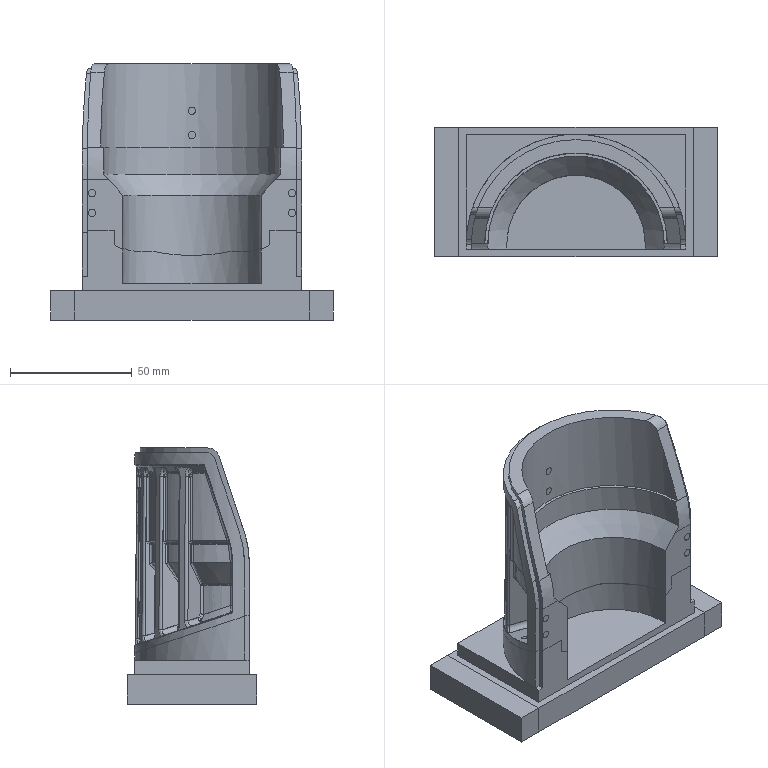NC program | NX | posted by the shop | part box 116 x 53 x 105 mm
Lines 1 to 928 of 572762:
CYCLE800
TRAFOOF
TRANS
ROT
G40 G17 G710 G94 G90 G60 G601 FNORM
TRAFOOF
SUPA G0 Z-1. D0
SUPA G0 X-1.0 Y-1.0
T18 M6
;(T18:C-D10  D=10. R=0.)
;(XY=0.mm Z=0.1mm)
G54 G90 D1
G0 A0.0 C=DC(0.0)
CYCLE832(0.12,_TOP_SURFACE_SMOOTH_ON+_ORI_SEMIFIN,1.)
G0 X54.1 Y-23.625 S7000 M3 M8
Z43.
Z3.1
G94 G1 Z.1 F1500.
X53.
X-53.
Y-15.75
X53.
Y-7.875
X-53.
Y0.0
X53.
Y7.875
X-53.
Y15.75
X53.
Y23.625
X-53.
X-54.1
Z3.1
G0 Z43.
CYCLE832()
;(T18:C-D10  D=10. R=0.)
;(XY=0.3mm Z=0.3mm)
SUPA G0 Z-1. D0
SUPA G0 X-1.0 Y-1.0
G54 G90 D1
CYCLE832(0.32,_ROUGH,1.)
TRAFOOF
CYCLE800(0,"AFMING",100000,57,0.,0.,0.,-90.,0.,-0.,0.,0.,0.,-1,100.,1)
G0 X55.844 Y85.217 S7000 M3
Z67.41
X55.844 Y85.217 Z67.41
Z3.8
G1 Z.8 F3500.
G3 X55.651 Y86.799 I-.713 J.7156
G1 X54.93 Y87.243
X54.186 Y87.648
G3 X52.997 Y87.1846 I-.31 J-.963
X52.447 Y81.73 I20.436 J-4.814
G1 X52.397 Y72.375
X52.369 Y1.951
G2 X48.396 Y-3.028 I-6.274 J.932
X41.431 Y-4.3 I-6.806 J17.567
G3 X39.312 Y-4.464 I-.547 J-6.7
G1 X38.261 Y-4.967
G3 X37.691 Y-6.068 I.414 J-.913
X38.403 Y-6.8609 Z1.081 I1.068 J.243 TURN=0
G1 X39.178 Y-7.242 Z1.3
X40.9306 Y-8.09 F15000.
X41.169 Y-8.126
X41.409 Y-8.116
X43.432 Y-7.734
X45.441 Y-7.287
G3 X48.546 Y-6.223 I-6.272 J23.35
G1 X51.559 Y-4.93
G3 X55.195 Y.607 I-3.082 J5.986
G1 X55.354 Y3.693
X55.433 Y6.781
X56.109 Y84.343
X55.986 Y84.715
X55.727 Y85.171
X54.75 Y86.892 Z.8 F3500.
G3 X54.225 Y87.552 I-1.461 J-.623
X52.968 Y87.361 I-.512 J-.861
X52.003 Y82.98 I9.95 J-4.489
X51.7982 Y72.298 I208.361 J-9.332
G1 X51.776 Y4.15
G2 X46.875 Y-2.259 I-7.688 J.8
X40.862 Y-3.6267 I-7.74 J20.124
G3 X39.209 Y-4.523 I.69 J-3.245
X38.928 Y-5.8101 I.597 J-.805
X39.845 Y-6.345 Z1.08 I.942 J.562 TURN=0
G1 X40.704 Y-6.475 Z1.3
X42.797 Y-6.781 F15000.
X43.0644 Y-6.749
X48.069 Y-5.4272
G3 X51.335 Y-3.4251 I-2.55 J7.826
G1 X52.151 Y-2.616
X52.926 Y-1.767
G3 X54.4545 Y1.9676 I-5.961 J4.62
X54.917 Y8.1208 I-45.709 J6.5262
G1 X55.097 Y83.6231
X54.875 Y85.1759
X54.6051 Y86.983 Z.838 F3500.
X54.55 Y87.124 Z.8
G3 X52.881 Y87.335 I-.903 J-.431
X51.5659 Y83.141 I7.417 J-4.629
X51.199 Y70.723 I125.865 J-9.938
G1 X51.161 Y5.775
G2 X45.553 Y-1.5865 I-8.669 J.787
X41.04 Y-3.01 I-24.116 J68.574
G3 X40.107 Y-3.859 I1.703 J-2.811
X39.802 Y-5.101 I.597 J-.805
X40.692 Y-5.6815 Z1.08 I.969 J.514 TURN=0
G1 X41.543 Y-5.854 Z1.3
X43.403 Y-6.221 F15000.
X43.692 Y-6.191
X43.963 Y-6.085
X49.2849 Y-2.953
G3 X52.679 Y.725 I-6.142 J9.073
X53.789 Y3.142 I-9.965 J6.04
G1 X53.966 Y3.937
X54.05 Y4.748
X54.156 Y7.837
X54.2243 Y10.926
X55.047 Y83.497
X54.802 Y85.18
X54.514 Y86.981 Z.839 F3500.
X54.456 Y87.124 Z.8
G3 X52.821 Y87.353 I-.896 J-.445
X51.177 Y83.411 I5.612 J-4.654
X50.615 Y73.095 I70.0607 J-8.9932
G1 X50.569 Y7.525
G2 X44.815 Y-.77 I-9.467 J.424
G1 X42.844 Y-1.662
G2 X40.805 Y-3.102 I-10.229 J12.317
G1 X40.655 Y-3.27
G3 X40.884 Y-4.794 I.746 J-.667
X41.802 Y-4.895 Z1.039 I.592 J1.162 TURN=0
G1 X42.826 Y-4.768 Z1.3
X44.706 Y-4.526 F15000.
X44.955 Y-4.422
G3 X48.058 Y-2.402 I-11.603 J21.212
G1 X50.369 Y-.546
G3 X52.6816 Y3.133 I-4.852 J5.616
X53.56 Y7.794 I-25.859 J7.289
G1 X53.633 Y9.199
X55.086 Y83.83
X54.7686 Y85.177
X54.288 Y87.0955 Z.8 F3500.
G3 X52.866 Y87.557 I-.917 J-.402
X50.885 Y83.959 I4.201 J-4.656
X50.0605 Y74.984 I42.887 J-8.467
G1 X49.998 Y66.826
X49.9665 Y8.951
G2 X44.667 Y.237 I-10.345 J.323
G3 X43.144 Y-1.352 I1.364 J-2.832
G1 X42.844 Y-1.662
G3 X43.3856 Y-3.342 I.719 J-.695
X44.258 Y-3.132 Z1.031 I.14 J1.335 TURN=0
G1 X45.214 Y-2.669 Z1.3
X46.966 Y-1.821 F15000.
X48.703 Y-.943
G3 X50.137 Y.509 I-2.2007 J3.607
G1 X51.6321 Y3.07
G3 X52.737 Y6.707 I-10.456 J5.162
G1 X52.898 Y8.242
X52.968 Y9.784
X53.953 Y83.3736
X54.083 Y85.165
X54.187 Y86.795 Z.887 F3500.
X54.095 Y87.125 Z.8
G3 X52.798 Y87.615 I-.904 J-.431
X50.563 Y84.212 I3.395 J-4.667
X49.516 Y75.745 I33.271 J-8.412
X49.398 Y63.5248 I611.077 J-11.991
G1 X49.367 Y10.35
G2 X45.447 Y1.972 I-11.0628 J.0696
G3 X44.13 Y.553 I2.872 J-3.987
G2 X43.6261 Y-.568 I-4.072 J1.158
G3 X43.988 Y-1.963 I.853 J-.524
X45.011 Y-1.957 Z1.069 I.506 J.97 TURN=0
G1 X45.8612 Y-1.625 Z1.3
X47.748 Y-.877 F15000.
X47.926 Y-.736
X48.078 Y-.568
X50.408 Y2.93
G3 X52.304 Y9.496 I-12.158 J7.068
G1 X53.771 Y83.349
X53.9585 Y85.177
X54.051 Y85.988 Z1.093 F3500.
X54.101 Y86.803 Z.887
X54.01 Y87.1328 Z.8
G3 X52.614 Y87.567 I-.901 J-.435
X50.225 Y84.351 I2.982 J-4.709
X48.98 Y76.204 I27.997 J-8.45
X48.798 Y62.1 I403.271 J-12.238
G1 X48.767 Y11.65
G2 X45.1621 Y2.856 I-13.09 J.231
G3 X44.293 Y1.462 I2.508 J-2.531
G1 X44.124 Y.529
G3 X44.849 Y-.686 I.971 J-.245
X45.862 Y-.385 Z1.079 I.232 J1.0738 TURN=0
G1 X46.551 Y.153 Z1.3
X48.326 Y1.556 F15000.
G3 X50.309 Y4.865 I-15.901 J11.776
X51.075 Y7.201 I-10.588 J4.766
X51.877 Y13.303 I-28.779 J6.887
G1 X53.01 Y83.391
X53.564 Y85.175
X53.988 Y86.567 Z.932 F3500.
X53.982 Y86.8268 Z.866
X53.922 Y87.08 Z.8
G3 X52.997 Y87.699 I-.927 J-.385
X50.979 Y86.405 I.371 J-2.8
X48.891 Y80.7036 I10.399 J-7.0413
X48.218 Y68.369 I88.071 J-10.989
G1 X48.169 Y12.9258
G2 X45.388 Y4.437 I-14.695 J.114
G3 X44.347 Y2.488 I4.572 J-3.693
G1 X44.292 Y1.444
G3 X44.953 Y.441 I1.001 J-.06
X45.992 Y.644 Z1.079 I.334 J1.046 TURN=0
G1 X46.727 Y1.114 Z1.3
X47.72 Y1.763 F15000.
G3 X48.055 Y2.452 I-.688 J.76
G1 X52.847 Y83.803
X52.913 Y84.106
X53.326 Y85.169
X53.6 Y85.851 Z1.114 F3500.
X53.833 Y86.547 Z.928
X53.837 Y86.8 Z.864
X53.784 Y87.047 Z.8
G3 X52.847 Y87.699 I-.94 J-.352
X50.747 Y86.506 I.228 J-2.847
X49.838 Y84.837 I2.45 J-2.416
X48.1816 Y79.188 I12.972 J-6.872
X47.605 Y65.162 I120.7863 J-11.987
G1 X47.567 Y14.0503
G2 X44.995 Y5.187 I-17.807 J.363
G3 X44.347 Y2.464 I3.144 J-2.187
X45.455 Y1.47 I1.001 J.001
X46.277 Y2.053 Z1.064 I-.158 J1.094 TURN=0
G1 X46.803 Y2.821 Z1.3
X47.6162 Y4.025 F15000.
X47.721 Y4.412
X52.643 Y83.955
X53.102 Y85.17
X53.376 Y85.852 Z1.114 F3500.
X53.608 Y86.548 Z.928
X53.612 Y86.801 Z.864
X53.5589 Y87.049 Z.8
G3 X52.622 Y87.699 I-.939 J-.353
X50.041 Y85.495 I.09 J-2.719
X50.88 Y84.092 I1.052 J-.324
X52.032 Y84.568 Z1.132 I.196 J1.1581 TURN=0
G1 X52.479 Y85.0572 Z1.3
X52.5854 Y85.174 F15000.
X52.991 Y85.607 Z1.15 F3500.
X53.359 Y86.072 Z.999
G3 X53.471 Y86.836 Z.8 I-.986 J.535 TURN=0
X52.397 Y87.699 I-1.076 J-.24
X50.259 Y86.411 I-.086 J-2.276
G1 X50.219 Y86.077
G3 X51.945 Y85.099 I1.0976 J-.075
G1 X52.936 Y85.807
G3 X52.172 Y87.698 I-.764 J.792
X50.25 Y86.536 I-.249 J-1.757
G1 X50.2298 Y86.236
G3 X52.015 Y85.3033 I1.098 J-.0746
G1 X52.691 Y85.864
G3 X51.872 Y87.698 I-.819 J.734
X50.248 Y86.5 I-.27 J-1.333
X52.139 Y87.568 I1.3048 J-.102
X50.313 Y86.986 I-.64 J-1.1444
G2 X48.967 Y83.429 I-6.462 J.4142
G3 X47.484 Y77.555 I14.984 J-6.905
X47.0012 Y62.695 I154.428 J-12.4597
G1 X46.965 Y15.1
G2 X44.635 Y5.965 I-21.638 J.653
G1 X44.347 Y5.098
Y3.598
G3 X46.545 Y3.536 I1.1 J0.
G1 X46.658 Y5.541
X46.769 Y7.517 Z1.3
X50.957 Y81.972 F15000.
X50.9927 Y82.52 Z1.161 F3500.
X50.99 Y83.068 Z1.022
G3 X50.536 Y83.794 Z.8 I-1.098 J-.182 TURN=0
X49.071 Y83.606 I-.628 J-.905
X47.379 Y79.8146 I5.919 J-4.916
X46.475 Y69.356 I56.897 J-10.182
G1 X46.399 Y58.275
X46.359 Y16.0001
G2 X44.364 Y6.962 I-26.36 J1.079
G1 X44.347 Y5.061
G3 X46.545 Y5.001 I1.1 J0.
G1 X46.5974 Y5.961
X46.705 Y7.937 Z1.3
X50.705 Y81.7157 F15000.
X50.739 Y82.264 Z1.161 F3500.
X50.736 Y82.813 Z1.022
G3 X50.282 Y83.537 Z.8 I-1.0978 J-.184 TURN=0
X48.943 Y83.474 I-.628 J-.9055
X47.063 Y80.18 I4.108 J-4.527
X45.938 Y70.643 I40.914 J-9.662
X45.799 Y56.325 I637.665 J-13.3519
G1 X45.758 Y16.975
G2 X44.184 Y8.359 I-31.504 J1.3038
G3 X44.3262 Y7.267 I5.283 J.134
G1 X44.335 Y6.742
G3 X46.472 Y6.393 I1.1 J.019
G1 X46.549 Y6.887 Z.927
X46.568 Y7.387 Z1.053
X46.618 Y8.362 Z1.3
X50.364 Y81.419 F15000.
X50.3966 Y81.971 Z1.16 F3500.
X50.392 Y82.524 Z1.02
G3 X49.943 Y83.243 Z.8 I-1.098 J-.186 TURN=0
X48.5993 Y83.184 I-.634 J-.902
X46.524 Y79.7 I4.14 J-4.826
X45.35 Y70.108 I40.181 J-9.7839
X45.199 Y56.25 I626.297 J-13.752
G1 X45.156 Y17.875
G2 X43.916 Y9.6902 I-38.899 J1.705
G3 X44.075 Y8.504 I1.546 J-.397
G1 X44.18 Y7.989
G3 X45.979 Y7.378 I1.078 J.219
X46.3695 Y8.4274 Z1.092 I-.918 J.939 TURN=0
G1 X46.409 Y9.245 Z1.3
X49.908 Y81.031 F15000.
X49.939 Y81.584 Z1.16 F3500.
X49.934 Y82.138 Z1.0191
G3 X49.486 Y82.855 Z.8 I-1.098 J-.188 TURN=0
X48.141 Y82.796 I-.634 J-.902
X45.9618 Y79.17 I4.266 J-5.032
X44.785 Y69.9959 I39.41 J-9.717
X44.6 Y54.975 I457.94 J-13.17
G1 X44.555 Y18.775
G2 X43.537 Y10.733 I-51.515 J2.439
G3 X43.942 Y8.81 I2.766 J-.422
X45.467 Y8.278 I1.009 J.44
X46.058 Y9.384 Z1.134 I-.578 J1.0195 TURN=0
G1 X46.088 Y10.037 Z1.3
X49.383 Y80.573 F15000.
X49.418 Y81.159 Z1.151 F3500.
X49.402 Y81.7468 Z1.002
G3 X48.988 Y82.412 Z.8 I-1.098 J-.222 TURN=0
X47.769 Y82.481 I-.662 J-.883
X45.723 Y79.622 I2.988 J-4.301
X44.315 Y71.537 I27.9197 J-9.026
X43.999 Y55.351 I273.069 J-13.4202
G1 X43.965 Y19.9759
G2 X43.098 Y11.541 I-74.422 J3.384
G3 X43.5717 Y9.661 I2.158 J-.456
X45.051 Y9.106 I1.009 J.44
X45.689 Y10.244 Z1.15 I-.533 J1.046 TURN=0
G1 X45.7172 Y10.8365 Z1.3
X49.071 Y80.3461 F15000.
X49.107 Y80.953 Z1.146 F3500.
X49.097 Y81.561 Z.992
G3 X48.725 Y82.206 Z.8 I-1.1066 J-.21 TURN=0
X47.588 Y82.375 I-.707 J-.849
X45.462 Y79.892 I2.144 J-3.987
X44.375 Y76.218 I16.1043 J-6.762
G2 X44.302 Y72.5245 I-59.855 J-.66
G3 X43.51 Y65.556 I27.897 J-6.698
G1 X43.429 Y55.97
X43.39 Y22.102
G2 X42.645 Y12.462 I-91.099 J2.188
G3 X42.8445 Y10.67 I3.454 J-.523
G1 X43.291 Y10.067
G3 X44.644 Y9.728 I.884 J.658
X45.2824 Y10.842 Z1.144 I-.52 J1.038 TURN=0
G1 X45.314 Y11.457 Z1.3
X48.86 Y80.24 F15000.
X48.898 Y80.853 Z1.145 F3500.
X48.892 Y81.466 Z.989
G3 X48.531 Y82.106 Z.8 I-1.11 J-.203 TURN=0
X47.3809 Y82.287 I-.721 J-.837
X45.042 Y79.776 I1.919 J-4.134
X44.346 Y77.437 I4.053 J-2.479
G1 X44.375 Y76.237
G3 X45.717 Y75.191 I1.1 J.027
X46.562 Y76.018 Z1.113 I-.292 J1.145 TURN=0
G1 X46.842 Y76.701 Z1.3
X48.164 Y79.927 F15000.
X48.3739 Y80.429 Z1.162 F3500.
X48.548 Y80.944 Z1.024
G3 X48.348 Y81.785 Z.8 I-1.097 J.184 TURN=0
X47.036 Y82.14 I-.883 J-.66
X44.346 Y78.9216 I1.9825 J-4.39
G1 X44.345 Y77.8716
G3 X45.56 Y76.777 I1.101 J0.
X46.503 Y77.521 Z1.119 I-.154 J1.165 TURN=0
G1 X46.835 Y78.156 Z1.3
X47.632 Y79.685 F15000.
X47.889 Y80.168 Z1.161 F3500.
X48.112 Y80.667 Z1.023
G3 X47.995 Y81.518 Z.8 I-1.075 J.286 TURN=0
X46.622 Y81.964 I-.944 J-.568
X44.346 Y79.569 I1.159 J-3.38
G1 X44.346 Y78.894
G3 X45.406 Y77.794 I1.101 J.001
X46.469 Y78.447 Z1.1321 I.01 J1.175 TURN=0
G1 X46.833 Y79. Z1.3
X47.185 Y79.5348 F15000.
X47.487 Y79.986 Z1.1624 F3500.
X47.757 Y80.457 Z1.0248
G3 X47.721 Y81.322 Z.8 I-1.041 J.391 TURN=0
X46.538 Y81.928 I-.992 J-.4802
X44.346 Y80.008 I.357 J-2.618
G1 X44.346 Y79.558
G3 X46.305 Y78.87 I1.1 J-0.
G1 X47.393 Y80.251
G3 X46.242 Y81.875 I-.958 J.541
X44.3465 Y80.357 I.109 J-2.0785
G1 X44.346 Y79.982
G3 X46.2922 Y79.278 I1.1 J-0.
G1 X47.015 Y80.17
G3 X45.873 Y81.809 I-.949 J.557
X44.3465 Y80.352 I-.013 J-1.514
X46.222 Y79.572 I1.1 J-0.
G1 X46.51 Y79.851
X46.7504 Y80.174
G3 X45.578 Y81.757 I-.98 J.5
X44.347 Y80.519 I-.033 J-1.198
X46.425 Y81.235 I1.157 J.015
X45.13 Y81.668 I-.955 J-.702
X44.357 Y80.759 I.259 J-1.003
G1 X44.381 Y73.756
G2 X43.624 Y70.485 I-8.189 J.172
G3 X42.896 Y62.834 I32.757 J-6.977
G1 X42.83 Y50.924
X42.782 Y22.325
G2 X42.413 Y16.147 I-96.39 J2.648
G1 X42.425 Y11.313
G3 X42.888 Y10.61 I3.131 J1.561
X44.259 Y10.279 I.884 J.657
X44.875 Y11.439 Z1.153 I-.547 J1.035 TURN=0
G1 X44.886 Y12.021 Z1.3
X45.9459 Y69.831 F15000.
X45.961 Y70.38 Z1.161 F3500.
X45.937 Y70.929 Z1.022
G3 X45.458 Y71.636 Z.8 I-1.0905 J-.223 TURN=0
X43.928 Y71.293 I-.595 J-.926
X42.814 Y68.266 I6.092 J-3.96
G1 X42.413 Y16.143
G3 X44.613 Y16.114 I1.1 J-.0084
G1 X45.068 Y40.888
X45.104 Y42.8661 Z1.3
X45.589 Y69.2706 F15000.
X45.604 Y69.8148 Z1.162 F3500.
X45.58 Y70.359 Z1.024
G3 X45.09 Y71.07 Z.8 I-1.089 J-.225 TURN=0
X43.571 Y70.72 I-.5851 J-.933
X42.84 Y69.279 I3.4509 J-2.656
X45.009 Y68.917 I1.09 J-.148
X43.604 Y70.3511 I-1.06 J.367
X42.819 Y68.82 I.56 J-1.2538
G1 X42.814 Y68.22
G3 X43.8292 Y67.2024 I1.011 J-.007
G1 X45.29 Y67.2098
Z3.8
G0 Z32.3
X47.05 Y79.524
Z4.3
G1 Z1.3
G3 X46.841 Y80.314 I-1.016 J.1536
G1 X46.371 Y80.912
X45.8713 Y81.485
G3 X45.031 Y81.684 I-.634 J-.8035
X44.164 Y80.417 I.526 J-1.29
X44.058 Y77.434 I14.471 J-2.0078
G2 X43.989 Y72.5245 I-29.045 J-2.0436
X42.9049 Y70.244 I-5.927 J1.419
G1 X42.825 Y69.559
G3 X45.0182 Y69.426 I1.1 J-.008
G1 X46.265 Y80.384
G3 X44.596 Y81.445 I-1.093 J.124
X44.058 Y79.7628 I1.285 J-1.338
X46.258 Y79.767 I1.1 J.0001
G1 X46.239 Y80.792
G3 X45.0572 Y81.703 I-1.085 J-.186
X44.058 Y80.445 I.153 J-1.148
X46.3563 Y80.661 I1.158 J.019
X44.983 Y81.693 I-1.206 J-.176
X44.073 Y80.788 I.105 J-1.015
X44.878 Y79.666 I1.003 J-.13
G1 X46.5677 Y79.33
Z4.3
G0 Z32.8
X46.715 Y79.447
Z4.8
G1 Z1.8
G3 X46.537 Y80.245 I-1.009 J.1937
G1 X46.089 Y80.866
X45.606 Y81.46
G3 X44.734 Y81.676 I-.657 J-.782
X43.877 Y80.414 I.538 J-1.288
X43.782 Y77.458 I13.196 J-1.905
G2 X43.668 Y72.5245 I-25.751 J-1.872
G3 X42.8369 Y70.356 I18.446 J-8.308
G1 X42.83 Y70.131
G3 X44.3326 Y69.237 I1. J-.029
G1 X44.648 Y69.52 Z1.907
X44.907 Y69.855 Z2.0145
X45.602 Y70.744 Z2.3
X46.5571 Y71.98 F15000.
X46.686 Y72.357
X47.46 Y78.4425
X47.402 Y78.744
X47.26 Y79.017
X46.933 Y79.4521
X45.745 Y81.034 Z1.8 F3500.
G3 X44.304 Y81.437 I-.916 J-.499
X43.7693 Y79.758 I1.288 J-1.335
X45.969 Y79.762 I1.1 J-0.
G1 X45.9498 Y80.79
G3 X44.768 Y81.7 I-1.085 J-.187
X43.769 Y80.441 I.157 J-1.15
X46.07 Y80.659 I1.159 J.018
X44.6938 Y81.689 I-1.2068 J-.177
X43.785 Y80.784 I.106 J-1.015
X44.535 Y79.675 I1.003 J-.13
G1 X46.28 Y79.2274
Z4.8
G0 Z33.3
X46.375 Y79.387
Z5.3
G1 Z2.3
G3 X46.23 Y80.139 I-1.015 J.195
G1 X45.811 Y80.797
X45.3522 Y81.426
G3 X44.449 Y81.674 I-.691 J-.749
X43.589 Y80.413 I.533 J-1.287
X43.481 Y78.67 I7.858 J-1.36
G1 X43.531 Y73.756
G2 X42.84 Y70.645 I-26.463 J4.24
G1 X42.839 Y70.57
G3 X44.105 Y69.583 I1. J-.022
X44.8009 Y70.15 Z2.531 I-.451 J1.264 TURN=0
G1 X45.462 Y70.98 Z2.8
X46.563 Y72.379 F15000.
X46.645 Y72.583
X46.695 Y72.796
X47.167 Y78.431
X47.106 Y78.711
X46.975 Y78.965
X46.65 Y79.407
X45.478 Y81.001 Z2.3 F3500.
G3 X44.165 Y81.51 I-.949 J-.5
X43.481 Y80.505 I.696 J-1.208
G1 X43.481 Y79.755
G3 X45.681 Y79.761 I1.1 J0.
G1 X45.66 Y80.789
G3 X44.482 Y81.697 I-1.085 J-.1885
X43.481 Y80.439 I.157 J-1.152
X45.784 Y80.655 I1.16 J.018
X44.408 Y81.687 I-1.208 J-.177
X43.497 Y80.782 I.104 J-1.015
X44.199 Y79.6859 I1.003 J-.13
G1 X45.993 Y79.131
Z5.3
G0 Z32.3
X44.888 Y14.219
Z4.3
G1 Z1.3
G2 X44.92 Y12.211 I.125 J-1.002
G1 X44.114 Y12.296
X43.305 Y12.337
G3 X42.439 Y11.1922 I.135 J-1.002
X43.259 Y9.73 I4.86 J1.763
G2 X44.0749 Y6.036 I-5.656 J-3.187
X43.999 Y1.1107 I-79.727 J-1.238
X42.872 Y-1.352 I-6.094 J1.301
X40.283 Y-3.3335 I-11.833 J12.779
X38.747 Y-4.575 I-3.513 J2.775
G3 X38.769 Y-6.377 I.445 J-.896
X39.611 Y-6.421 Z1.516 I.488 J1.2757 TURN=0
G1 X40.72 Y-6.262 Z1.8
X42.639 Y-5.975 F15000.
X42.855 Y-5.871
X43.048 Y-5.728
X45.194 Y-3.595
X47.317 Y-1.438
G3 X47.994 Y.4562 I-2.322 J1.899
G1 X47.944 Y1.689
X47.807 Y2.915
X46.671 Y10.232
G3 X46.2299 Y10.7949 I-.9839 J-.316
G1 X45.115 Y11.464
X44.427 Y11.889 Z1.595 F3500.
X43.717 Y12.273 Z1.391
X43.362 Y12.3271 Z1.3
G3 X42.403 Y11.242 I.0387 J-1.
X42.647 Y10.658 I4.631 J1.596
X43.541 Y10.205 I.847 J.563
G1 X44.037 Y10.222
X44.531 Y10.284
G3 X45.244 Y11.216 I-.299 J.9682
G1 Z4.3
G0 Z32.8
X44.884 Y13.868
Z4.8
G1 Z1.8
G2 X44.797 Y11.878 I.125 J-1.002
G1 X44.114 Y12.0328
X43.422 Y12.144
G3 X42.494 Y10.798 I.026 J-1.01
G1 X43.527 Y8.498
G2 X43.803 Y6.036 I-7.214 J-2.056
X43.727 Y1.1107 I-79.725 J-1.2383
X40.391 Y-2.959 I-5.332 J.9689
X38.3059 Y-4.635 I-5.396 J4.576
G3 X37.87 Y-5.143 I.55 J-.912
G1 X37.351 Y-6.4765
G3 X39.2996 Y-6.918 I.941 J-.366
G1 Z4.8
G0 Z33.3
X44.8894 Y13.903
Z5.3
G1 Z2.3
G2 X44.929 Y11.893 I.118 J-1.003
G1 X43.486 Y12.005
G3 X42.4 Y10.923 I-.077 J-1.008
X42.844 Y9.432 I3.671 J.2806
G2 X43.531 Y6.036 I-5.8103 J-2.943
X43.454 Y1.1107 I-76.611 J-1.27
X40.2801 Y-2.9 I-5.4618 J1.061
X37.841 Y-4.834 I-25.176 J29.243
G1 X37.075 Y-6.452
G3 X39.005 Y-6.937 I.923 J-.411
G1 Z5.3
G0 Z31.8
X-37.729 Y-7.656
Z3.8
G1 Z.8
X-37.678 Y-5.922
G3 X-38.301 Y-4.959 I-1.013 J.027
X-44.141 Y-4.44 I-5.062 J-23.823
G2 X-47.661 Y-3.969 I-.679 J8.318
X-51.5736 Y1.093 I3.505 J6.752
X-52.363 Y8.906 I30.532 J7.032
G1 X-52.4249 Y86.492
G3 X-52.633 Y87.253 I-2.235 J-.202
X-54.39 Y86.981 I-.804 J-.617
G1 X-55.316 Y85.232 Z1.3
X-55.729 Y84.423 F15000.
X-55.781 Y84.105
Y8.663
G3 X-54.881 Y1.354 I30.223 J.01
G1 X-54.148 Y-1.518
G3 X-51.704 Y-5.099 I6.794 J2.011
G1 X-49.6603 Y-6.611
G3 X-46.299 Y-7.749 I3.891 J5.958
G1 X-43.792 Y-7.941
X-41.283 Y-8.106
X-40.963 Y-8.021
X-39.275 Y-7.256
X-38.112 Y-6.7124 Z.975 F3500.
G3 X-37.714 Y-6.1608 Z.8 I-.613 J.861 TURN=0
X-38.301 Y-4.959 I-.963 J.273
X-42.346 Y-4.022 I-4.215 J-8.995
G2 X-46.978 Y-2.8728 I-.191 J9.139
X-51.05 Y3.459 I5.553 J8.048
X-51.773 Y12.488 I43.506 J8.025
G1 X-51.836 Y85.291
G3 X-52.466 Y87.406 I-3.628 J.07
X-54.027 Y87.204 I-.701 J-.714
G1 X-54.192 Y86.927
X-55.2024 Y85.2258 Z1.3
X-55.411 Y84.885 F15000.
X-55.579 Y84.523
X-55.614 Y84.258
Y18.71
G3 X-54.598 Y6.427 I74.886 J.014
G1 X-53.856 Y2.064
G3 X-51.873 Y-2.97 I15.385 J3.15
X-49.599 Y-5.153 I6.075 J4.054
G1 X-46.967 Y-6.737
G3 X-43.815 Y-7.692 I3.993 J7.504
G1 X-41.758 Y-7.884
X-41.554 Y-7.846
X-41.356 Y-7.781
X-39.775 Y-6.997
X-38.635 Y-6.415 Z.976 F3500.
G3 X-38.256 Y-5.846 Z.8 I-.643 J.838 TURN=0
X-38.7495 Y-4.732 I-.9746 J.234
X-42.792 Y-3.5 I-5.06 J-9.357
G2 X-49.86 Y2.972 I1.991 J9.27
X-51.092 Y11.097 I26.204 J8.131
X-51.199 Y23.846 I622.914 J11.562
G1 X-51.236 Y84.035
G3 X-52.139 Y87.387 I-6.059 J.165
G1 X-52.252 Y87.485
G3 X-53.75 Y87.1575 I-.612 J-.792
G1 X-53.898 Y86.661 Z.931
X-53.992 Y86.152 Z1.062
X-54.177 Y85.229 Z1.3
X-54.348 Y84.433 F15000.
X-54.478 Y83.629
X-54.466 Y7.6957
G3 X-53.384 Y3.418 I12.434 J.87
G1 X-51.72 Y-.365
G3 X-47.854 Y-5.077 I12.419 J6.247
X-45.214 Y-6.215 I3.831 J5.258
G1 X-43.182 Y-6.579
X-40.977 Y-6.339
X-39.676 Y-6.176 Z.968 F3500.
G3 X-39.141 Y-5.8 Z.8 I-.315 J1.016 TURN=0
X-39.474 Y-4.337 I-.812 J.584
X-42.388 Y-3.082 I-5.573 J-8.929
G2 X-49.441 Y4.739 I3.841 J10.554
X-50.526 Y13.874 I35.114 J8.803
G1 X-50.598 Y25.7234
X-50.638 Y82.929
G3 X-51.636 Y87.138 I-8.206 J.2772
G1 X-51.987 Y87.522
G3 X-53.439 Y87.148 I-.561 J-.829
G1 X-53.608 Y86.567 Z.953
X-53.73 Y85.973 Z1.106
X-53.894 Y85.225 Z1.3
X-54.073 Y84.449 F15000.
X-54.213 Y83.666
Y20.592
G3 X-53.196 Y8.309 I74.886 J.014
G1 X-52.454 Y3.945
G3 X-50.507 Y-1.018 I15.2646 J3.124
X-48.117 Y-3.414 I6.9951 J4.588
G1 X-45.805 Y-4.942
X-43.481 Y-6.449
G3 X-42.847 Y-6.51 I.413 J.968
G1 X-41.273 Y-6.144
X-40.016 Y-5.837 Z.972 F3500.
G3 X-39.5211 Y-5.385 Z.8 I-.431 J.968 TURN=0
X-39.767 Y-4.145 I-.885 J.469
X-42.86 Y-2.265 I-11.2507 J-15.026
G2 X-49.069 Y6.7 I6.912 J11.4201
X-49.954 Y16.768 I49.061 J9.387
G1 X-50.0322 Y81.692
G3 X-51.025 Y86.7335 I-11.417 J.37
X-51.707 Y87.553 I-2.903 J-1.724
X-53.091 Y87.134 I-.492 J-.872
G1 X-53.327 Y86.325 Z1.013
X-53.519 Y85.504 Z1.226
X-53.589 Y85.221 Z1.3
X-53.926 Y83.817 F15000.
X-53.933 Y30.517
G3 X-52.977 Y13.256 I156.702 J.022
G1 X-52.294 Y7.24
G3 X-50.705 Y1.449 I24.478 J3.602
G1 X-50.264 Y.36
X-49.761 Y-.7004
G3 X-47.751 Y-2.823 I5.475 J3.171
G1 X-44.332 Y-5.041
X-44.033 Y-5.123
X-42.153 Y-5.336
X-40.8652 Y-5.467 Z.972 F3500.
G3 X-40.248 Y-5.205 Z.8 I-.083 J1.056 TURN=0
X-40.167 Y-3.814 I-.677 J.737
X-42.173 Y-2.261 I-5.9121 J-5.565
G2 X-48.712 Y8.926 I9.918 J13.301
X-49.379 Y20.295 I74.847 J10.093
G1 X-49.441 Y80.933
G3 X-50.449 Y86.382 I-13.61 J.2984
X-51.46 Y87.601 I-2.684 J-1.1974
X-52.789 Y87.122 I-.424 J-.907
G1 X-53.322 Y85.217 Z1.3
X-53.677 Y83.877 F15000.
X-53.686 Y40.459
G3 X-52.678 Y18.243 I245.95 J.026
G1 X-51.902 Y9.838
G3 X-49.892 Y1.745 I32.508 J3.7767
X-47.71 Y-1.546 I10.332 J4.483
G1 X-44.603 Y-4.782
X-44.345 Y-4.924
X-44.058 Y-4.99
X-42.356 Y-5.106
X-41.066 Y-5.179 Z.973 F3500.
G3 X-40.459 Y-4.8892 Z.8 I-.13 J1.051 TURN=0
X-40.412 Y-3.531 I-.712 J.704
X-41.689 Y-2.583 I-2.197 J-1.626
G2 X-43.646 Y-.622 I2.885 J4.837
X-48.42 Y12.231 I18.637 J14.236
X-48.795 Y26.396 I167.17 J11.5114
G1 X-48.837 Y79.9002
G3 X-49.263 Y83.861 I-14.975 J.394
G2 X-50.349 Y86.5137 I6.055 J4.028
G3 X-51.251 Y87.615 I-1.962 J-.687
X-52.543 Y86.119 I-.406 J-.955
G1 X-52.035 Y85.3181
G3 X-50.217 Y86.0685 I.783 J.681
X-51.357 Y87.699 I-1.53 J.144
G1 X-53.007 Y87.699
G3 X-53.205 Y85.517 I-0. J-1.1
G1 X-51.352 Y85.194
G3 X-50.237 Y86.368 I.016 J1.1006
X-51.372 Y87.699 I-1.171 J.151
X-50.276 Y86.804 I.005 J-1.112
X-51.188 Y87.685 I-1.017 J-.141
X-52.245 Y87.058 I-.124 J-.995
G1 X-52.958 Y85.212 Z1.3
X-53.386 Y84.083 F15000.
X-53.415 Y83.829
X-52.83 Y45.907
G3 X-52.0219 Y23.251 I787.657 J16.759
G1 X-51.746 Y17.582
X-51.4358 Y11.915
G3 X-50.117 Y4.053 I43.951 J3.33
X-48.881 Y.994 I16.291 J4.805
G1 X-47.719 Y-1.194
X-47.5089 Y-1.401
X-47.25 Y-1.544
X-45.575 Y-2.146
X-44.96 Y-2.374 Z1.134 F3500.
X-44.331 Y-2.564 Z.967
G3 X-43.693 Y-2.431 Z.8 I.119 J1.03 TURN=0
X-43.3453 Y-1.068 I-.516 J.858
G2 X-45.004 Y2.36 I26.9785 J15.17
X-47.954 Y14.833 I29.15 J13.48
X-48.197 Y31.253 I314.1472 J12.854
G1 X-48.239 Y79.078
G3 X-48.676 Y83.144 I-15.942 J.341
G1 X-49.334 Y83.971
G3 X-50.73 Y84.196 I-.811 J-.587
X-51.1532 Y83.239 Z1.076 I.676 J-.871 TURN=0
G1 X-51.198 Y82.354 Z1.3
X-51.282 Y80.597 F15000.
X-47.668 Y.813
G3 X-47.283 Y.202 I1.01 J.21
G1 X-46.405 Y-.45
X-45.337 Y-1.2259 Z.966 F3500.
G3 X-44.697 Y-1.319 Z.8 I.467 J.959 TURN=0
X-43.923 Y-.049 I-.184 J.984
X-46.085 Y7.052 I-678.9509 J-202.905
G2 X-47.517 Y19.691 I53.136 J12.418
G1 X-47.597 Y32.441
X-47.626 Y77.7579
G3 X-48.117 Y82.561 I-17.946 J.593
X-48.856 Y83.398 I-3.591 J-2.425
X-50.078 Y83.531 I-.697 J-.721
X-50.5662 Y82.585 Z1.0808 I.607 J-.912 TURN=0
G1 X-50.649 Y81.724 Z1.3
X-50.804 Y80.024 F15000.
X-47.629 Y2.922
X-47.5642 Y2.727
X-47.476 Y2.542
X-46.793 Y1.525
X-46.3925 Y.9127 Z1.115 F3500.
X-45.955 Y.326 Z.929
X-45.748 Y.177 Z.865
X-45.512 Y.079 Z.8
G3 X-44.271 Y1.1107 I.243 J.97
X-45.266 Y6.253 I-23.506 J-1.883
G2 X-46.924 Y20.901 I61.669 J14.3965
G1 X-46.996 Y33.501
X-47.036 Y77.367
G3 X-47.528 Y81.923 I-18.206 J.342
X-48.324 Y82.882 I-1.551 J-.478
X-49.669 Y83.028 I-.766 J-.792
X-50.181 Y81.862 Z1.14 I.638 J-.975 TURN=0
G1 X-50.152 Y81.2328 Z1.3
X-46.78 Y7.506 F15000.
X-46.689 Y5.529 Z.8 F3500.
X-46.61 Y3.618
X-46.5 Y1.71
G3 X-44.326 Y2.009 I1.075 J.231
X-45.145 Y8.368 I-29.572 J-.5741
G2 X-46.3683 Y24.726 I91.624 J15.077
G1 X-46.441 Y76.7603
G3 X-47.086 Y81.736 I-15.659 J.4996
X-48.026 Y82.6664 I-1.756 J-.833
X-49.262 Y82.6573 I-.611 J-.919
X-49.728 Y81.514 Z1.1284 I.697 J-.951 TURN=0
G1 X-49.701 Y80.837 Z1.3
X-46.733 Y7.8675 F15000.
X-46.653 Y5.89 Z.8 F3500.
X-46.602 Y4.492
X-46.524 Y3.094
G3 X-44.347 Y3.317 I1.077 J.223
X-44.983 Y11.135 I-43.072 J.431
G2 X-45.788 Y28.88 I143.876 J15.414
G1 X-45.8399 Y75.9389
G3 X-46.542 Y81.322 I-17.072 J.51
X-47.584 Y82.372 I-1.544 J-.489
X-48.698 Y82.28 I-.479 J-.9966
X-49.156 Y81.147 Z1.1246 I.714 J-.948 TURN=0
G1 X-49.132 Y80.455 Z1.3
X-46.643 Y8.3174 F15000.
X-46.574 Y6.34 Z.8 F3500.
X-46.525 Y5.351
G3 X-44.347 Y5.567 I1.078 J.2165
X-44.745 Y14.703 I-61.168 J1.914
G2 X-45.194 Y34.268 I265.761 J15.897
G1 X-45.231 Y74.83
G3 X-45.917 Y80.723 I-21.08 J.535
X-47.242 Y82.2063 I-1.912 J-.374
X-48.393 Y82.0876 I-.479 J-.996
X-48.815 Y80.994 Z1.11 I.75 J-.918 TURN=0
G1 X-48.7911 Y80.244 Z1.3
X-46.5457 Y8.793 F15000.
X-46.531 Y8.003 Z1.1 F3500.
X-46.467 Y7.216 Z.9
X-46.305 Y6.856 Z.8
G3 X-44.3262 Y7.267 I.901 J.631
X-44.059 Y12.901 I-17.771 J3.668
G2 X-44.595 Y36.565 I334.039 J19.405
G1 X-44.628 Y73.867
G3 X-45.335 Y80.255 I-23.845 J.596
X-46.513 Y81.96 I-2.4987 J-.467
G1 X-46.946 Y82.082
G3 X-47.958 Y81.861 I-.296 J-1.068
X-48.339 Y80.811 Z1.094 I.795 J-.882 TURN=0
G1 X-48.315 Y79.997 Z1.3
X-46.309 Y9.586 F15000.
X-46.297 Y8.954 Z1.14 F3500.
X-46.244 Y8.3234 Z.98
G3 X-45.871 Y7.733 Z.8 I1.101 J.283 TURN=0
X-44.102 Y8.369 I.6906 J.856
X-43.569 Y13.073 I-11.8227 J3.721
G2 X-43.994 Y38.143 I513.359 J21.248
G1 X-44.035 Y71.641
G2 X-44.382 Y73.756 I4.9497 J1.9
G3 X-44.617 Y79.144 I-27.9 J1.484
X-45.883 Y81.738 I-4.3895 J-.537
G1 X-46.525 Y81.964
G3 X-47.679 Y81.595 I-.297 J-1.063
X-47.8157 Y80.399 Z1.12 I.933 J-.713 TURN=0
G1 X-47.598 Y79.721 Z1.3
X-46.864 Y77.438 F15000.
X-46.66 Y76.775 Z1.124 F3500.